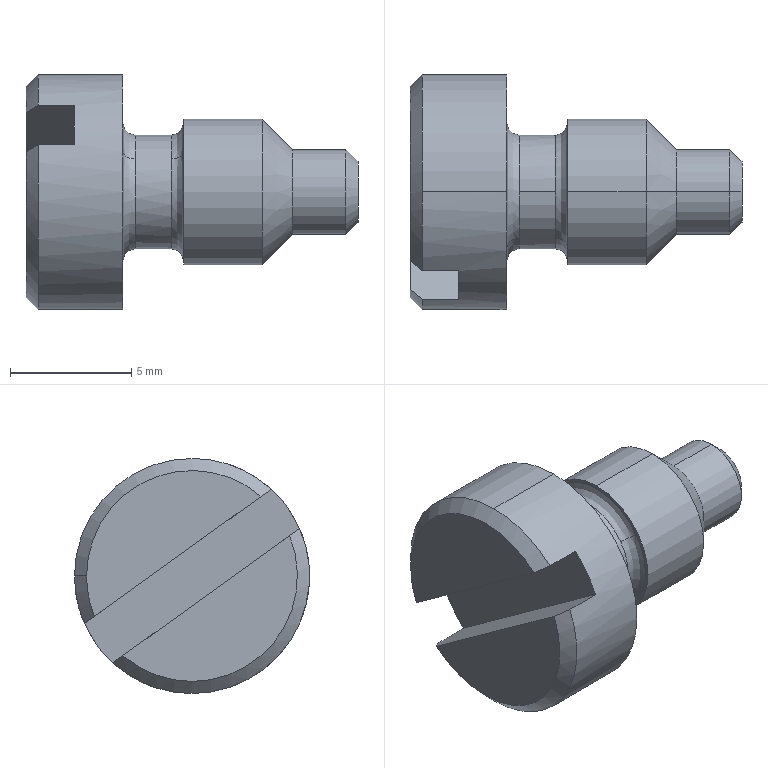Part | SolidWorks | features BaseBody 1 | 1 solid | 27 faces | box 13.7 x 9.7 x 9.7 mm | volume 438.23 mm3 | cylinder 8 | plane 8 | cone 7 | spline 4 | commonest cylinder face diameters 3.5 x2 4.7 x2 6 x2 9.7 x2
STEP:
#1=CARTESIAN_POINT('',(-26.901,-34.08,-0.15));
#2=VERTEX_POINT('',#1);
#3=CARTESIAN_POINT('',(-26.901,-34.08,-9.85));
#4=VERTEX_POINT('',#3);
#5=CARTESIAN_POINT('',(-26.901,-34.08,-5.));
#6=DIRECTION('',(-1.,0.,0.));
#7=DIRECTION('',(0.,0.,1.));
#8=AXIS2_PLACEMENT_3D('',#5,#6,#7);
#9=CIRCLE('',#8,4.85);
#10=EDGE_CURVE('',#2,#4,#9,.T.);
#11=ORIENTED_EDGE('',*,*,#10,.T.);
#12=CARTESIAN_POINT('',(-30.401,-34.08,-9.85));
#13=VERTEX_POINT('',#12);
#14=CARTESIAN_POINT('',(-26.901,-34.08,-9.85));
#15=DIRECTION('',(-1.,0.,0.));
#16=VECTOR('',#15,1000.);
#17=LINE('',#14,#16);
#18=EDGE_CURVE('',#4,#13,#17,.T.);
#19=ORIENTED_EDGE('',*,*,#18,.T.);
#20=CARTESIAN_POINT('',(-30.401,-30.814,-8.586));
#21=VERTEX_POINT('',#20);
#22=CARTESIAN_POINT('',(-30.401,-34.08,-5.));
#23=DIRECTION('',(1.,0.,0.));
#24=DIRECTION('',(0.,0.,1.));
#25=AXIS2_PLACEMENT_3D('',#22,#23,#24);
#26=CIRCLE('',#25,4.85);
#27=EDGE_CURVE('',#13,#21,#26,.T.);
#28=ORIENTED_EDGE('',*,*,#27,.T.);
#29=CARTESIAN_POINT('',(-28.901,-30.814,-8.586));
#30=VERTEX_POINT('',#29);
#31=CARTESIAN_POINT('',(-29.901,-30.814,-8.586));
#32=DIRECTION('',(-1.,0.,0.));
#33=VECTOR('',#32,1000.);
#34=LINE('',#31,#33);
#35=EDGE_CURVE('',#30,#21,#34,.T.);
#36=ORIENTED_EDGE('',*,*,#35,.F.);
#37=CARTESIAN_POINT('',(-28.901,-29.645,-6.963));
#38=VERTEX_POINT('',#37);
#39=CARTESIAN_POINT('',(-28.901,-34.08,-5.));
#40=DIRECTION('',(1.,0.,0.));
#41=DIRECTION('',(0.,0.,1.));
#42=AXIS2_PLACEMENT_3D('',#39,#40,#41);
#43=CIRCLE('',#42,4.85);
#44=EDGE_CURVE('',#30,#38,#43,.T.);
#45=ORIENTED_EDGE('',*,*,#44,.T.);
#46=CARTESIAN_POINT('',(-30.401,-29.645,-6.963));
#47=VERTEX_POINT('',#46);
#48=CARTESIAN_POINT('',(-29.901,-29.645,-6.963));
#49=DIRECTION('',(-1.,0.,0.));
#50=VECTOR('',#49,1000.);
#51=LINE('',#48,#50);
#52=EDGE_CURVE('',#38,#47,#51,.T.);
#53=ORIENTED_EDGE('',*,*,#52,.T.);
#54=CARTESIAN_POINT('',(-30.401,-29.23,-5.));
#55=VERTEX_POINT('',#54);
#56=CARTESIAN_POINT('',(-30.401,-34.08,-5.));
#57=DIRECTION('',(1.,0.,0.));
#58=DIRECTION('',(0.,0.,1.));
#59=AXIS2_PLACEMENT_3D('',#56,#57,#58);
#60=CIRCLE('',#59,4.85);
#61=EDGE_CURVE('',#47,#55,#60,.T.);
#62=ORIENTED_EDGE('',*,*,#61,.T.);
#63=CARTESIAN_POINT('',(-30.401,-34.08,-0.15));
#64=VERTEX_POINT('',#63);
#65=CARTESIAN_POINT('',(-30.401,-34.08,-5.));
#66=DIRECTION('',(1.,0.,0.));
#67=DIRECTION('',(0.,0.,1.));
#68=AXIS2_PLACEMENT_3D('',#65,#66,#67);
#69=CIRCLE('',#68,4.85);
#70=EDGE_CURVE('',#55,#64,#69,.T.);
#71=ORIENTED_EDGE('',*,*,#70,.T.);
#72=CARTESIAN_POINT('',(-26.901,-34.08,-0.15));
#73=DIRECTION('',(-1.,0.,0.));
#74=VECTOR('',#73,1000.);
#75=LINE('',#72,#74);
#76=EDGE_CURVE('',#2,#64,#75,.T.);
#77=ORIENTED_EDGE('',*,*,#76,.F.);
#78=EDGE_LOOP('',(#11,#19,#28,#36,#45,#53,#62,#71,#77));
#79=FACE_OUTER_BOUND('',#78,.T.);
#80=CARTESIAN_POINT('',(-26.901,-34.08,-5.));
#81=DIRECTION('',(-1.,0.,0.));
#82=DIRECTION('',(0.,0.,1.));
#83=AXIS2_PLACEMENT_3D('',#80,#81,#82);
#84=CYLINDRICAL_SURFACE('',#83,4.85);
#85=ADVANCED_FACE('',(#79),#84,.T.);
#86=CARTESIAN_POINT('',(-30.901,-30.061,-6.664));
#87=VERTEX_POINT('',#86);
#88=CARTESIAN_POINT('',(-30.901,-29.73,-5.));
#89=VERTEX_POINT('',#88);
#90=CARTESIAN_POINT('',(-30.901,-34.08,-5.));
#91=DIRECTION('',(1.,0.,0.));
#92=DIRECTION('',(0.,1.,0.));
#93=AXIS2_PLACEMENT_3D('',#90,#91,#92);
#94=CIRCLE('',#93,4.35);
#95=EDGE_CURVE('',#87,#89,#94,.T.);
#96=ORIENTED_EDGE('',*,*,#95,.T.);
#97=CARTESIAN_POINT('',(-30.401,-29.23,-5.));
#98=DIRECTION('',(0.7071,0.7071,0.));
#99=VECTOR('',#98,1000.);
#100=LINE('',#97,#99);
#101=EDGE_CURVE('',#89,#55,#100,.T.);
#102=ORIENTED_EDGE('',*,*,#101,.T.);
#103=ORIENTED_EDGE('',*,*,#61,.F.);
#104=CARTESIAN_POINT('',(-30.401,-29.645,-6.963));
#105=CARTESIAN_POINT('',(-30.568,-29.784,-6.863));
#106=CARTESIAN_POINT('',(-30.735,-29.922,-6.764));
#107=CARTESIAN_POINT('',(-30.901,-30.061,-6.664));
#108=B_SPLINE_CURVE_WITH_KNOTS('',3,(#104,#105,#106,#107),.UNSPECIFIED.,.F.,.F.,(4,4),(0.,0.0007159),.UNSPECIFIED.);
#109=EDGE_CURVE('',#47,#87,#108,.T.);
#110=ORIENTED_EDGE('',*,*,#109,.T.);
#111=EDGE_LOOP('',(#96,#102,#103,#110));
#112=FACE_OUTER_BOUND('',#111,.T.);
#113=CARTESIAN_POINT('',(-30.401,-34.08,-5.));
#114=DIRECTION('',(1.,0.,0.));
#115=DIRECTION('',(0.,1.,0.));
#116=AXIS2_PLACEMENT_3D('',#113,#114,#115);
#117=CONICAL_SURFACE('',#116,4.85,0.7854);
#118=ADVANCED_FACE('',(#112),#117,.T.);
#119=CARTESIAN_POINT('',(-24.901,-32.174,-6.374));
#120=VERTEX_POINT('',#119);
#121=CARTESIAN_POINT('',(-24.901,-34.08,-7.35));
#122=VERTEX_POINT('',#121);
#123=CARTESIAN_POINT('',(-24.901,-34.08,-5.));
#124=DIRECTION('',(-1.,0.,0.));
#125=DIRECTION('',(0.,0.,1.));
#126=AXIS2_PLACEMENT_3D('',#123,#124,#125);
#127=CIRCLE('',#126,2.35);
#128=EDGE_CURVE('',#120,#122,#127,.T.);
#129=ORIENTED_EDGE('',*,*,#128,.T.);
#130=CARTESIAN_POINT('',(-26.401,-34.08,-7.35));
#131=VERTEX_POINT('',#130);
#132=CARTESIAN_POINT('',(-24.901,-34.08,-7.35));
#133=DIRECTION('',(-1.,0.,0.));
#134=VECTOR('',#133,1000.);
#135=LINE('',#132,#134);
#136=EDGE_CURVE('',#122,#131,#135,.T.);
#137=ORIENTED_EDGE('',*,*,#136,.T.);
#138=CARTESIAN_POINT('',(-26.401,-32.174,-6.374));
#139=VERTEX_POINT('',#138);
#140=CARTESIAN_POINT('',(-26.401,-34.08,-5.));
#141=DIRECTION('',(1.,-0.000000001,-0.000000001));
#142=DIRECTION('',(0.,0.8113,-0.5846));
#143=AXIS2_PLACEMENT_3D('',#140,#141,#142);
#144=CIRCLE('',#143,2.35);
#145=EDGE_CURVE('',#131,#139,#144,.T.);
#146=ORIENTED_EDGE('',*,*,#145,.T.);
#147=CARTESIAN_POINT('',(-26.401,-31.73,-5.));
#148=VERTEX_POINT('',#147);
#149=CARTESIAN_POINT('',(-26.401,-34.08,-5.));
#150=DIRECTION('',(1.,0.,0.));
#151=DIRECTION('',(0.,0.,1.));
#152=AXIS2_PLACEMENT_3D('',#149,#150,#151);
#153=CIRCLE('',#152,2.35);
#154=EDGE_CURVE('',#139,#148,#153,.T.);
#155=ORIENTED_EDGE('',*,*,#154,.T.);
#156=CARTESIAN_POINT('',(-26.401,-34.08,-2.65));
#157=VERTEX_POINT('',#156);
#158=CARTESIAN_POINT('',(-26.401,-34.08,-5.));
#159=DIRECTION('',(1.,0.,0.000000001));
#160=DIRECTION('',(0.,-0.8113,0.5846));
#161=AXIS2_PLACEMENT_3D('',#158,#159,#160);
#162=CIRCLE('',#161,2.35);
#163=EDGE_CURVE('',#148,#157,#162,.T.);
#164=ORIENTED_EDGE('',*,*,#163,.T.);
#165=CARTESIAN_POINT('',(-24.901,-34.08,-2.65));
#166=VERTEX_POINT('',#165);
#167=CARTESIAN_POINT('',(-24.901,-34.08,-2.65));
#168=DIRECTION('',(-1.,0.,0.));
#169=VECTOR('',#168,1000.);
#170=LINE('',#167,#169);
#171=EDGE_CURVE('',#166,#157,#170,.T.);
#172=ORIENTED_EDGE('',*,*,#171,.F.);
#173=CARTESIAN_POINT('',(-24.901,-34.08,-5.));
#174=DIRECTION('',(-1.,0.,0.));
#175=DIRECTION('',(0.,0.,1.));
#176=AXIS2_PLACEMENT_3D('',#173,#174,#175);
#177=CIRCLE('',#176,2.35);
#178=EDGE_CURVE('',#166,#120,#177,.T.);
#179=ORIENTED_EDGE('',*,*,#178,.T.);
#180=EDGE_LOOP('',(#129,#137,#146,#155,#164,#172,#179));
#181=FACE_OUTER_BOUND('',#180,.T.);
#182=CARTESIAN_POINT('',(-24.901,-34.08,-5.));
#183=DIRECTION('',(-1.,0.,0.));
#184=DIRECTION('',(0.,0.,1.));
#185=AXIS2_PLACEMENT_3D('',#182,#183,#184);
#186=CYLINDRICAL_SURFACE('',#185,2.35);
#187=ADVANCED_FACE('',(#181),#186,.T.);
#188=CARTESIAN_POINT('',(-21.151,-34.08,-2.));
#189=VERTEX_POINT('',#188);
#190=CARTESIAN_POINT('',(-21.151,-34.08,-8.));
#191=VERTEX_POINT('',#190);
#192=CARTESIAN_POINT('',(-21.151,-34.08,-5.));
#193=DIRECTION('',(-1.,0.,0.));
#194=DIRECTION('',(0.,0.,1.));
#195=AXIS2_PLACEMENT_3D('',#192,#193,#194);
#196=CIRCLE('',#195,3.);
#197=EDGE_CURVE('',#189,#191,#196,.T.);
#198=ORIENTED_EDGE('',*,*,#197,.T.);
#199=CARTESIAN_POINT('',(-24.401,-34.08,-8.));
#200=VERTEX_POINT('',#199);
#201=CARTESIAN_POINT('',(-21.151,-34.08,-8.));
#202=DIRECTION('',(-1.,0.,0.));
#203=VECTOR('',#202,1000.);
#204=LINE('',#201,#203);
#205=EDGE_CURVE('',#191,#200,#204,.T.);
#206=ORIENTED_EDGE('',*,*,#205,.T.);
#207=CARTESIAN_POINT('',(-24.401,-34.08,-2.));
#208=VERTEX_POINT('',#207);
#209=CARTESIAN_POINT('',(-24.401,-34.08,-5.));
#210=DIRECTION('',(1.,0.,0.));
#211=DIRECTION('',(0.,0.,1.));
#212=AXIS2_PLACEMENT_3D('',#209,#210,#211);
#213=CIRCLE('',#212,3.);
#214=EDGE_CURVE('',#200,#208,#213,.T.);
#215=ORIENTED_EDGE('',*,*,#214,.T.);
#216=CARTESIAN_POINT('',(-21.151,-34.08,-2.));
#217=DIRECTION('',(-1.,0.,0.));
#218=VECTOR('',#217,1000.);
#219=LINE('',#216,#218);
#220=EDGE_CURVE('',#189,#208,#219,.T.);
#221=ORIENTED_EDGE('',*,*,#220,.F.);
#222=EDGE_LOOP('',(#198,#206,#215,#221));
#223=FACE_OUTER_BOUND('',#222,.T.);
#224=CARTESIAN_POINT('',(-21.151,-34.08,-5.));
#225=DIRECTION('',(-1.,0.,0.));
#226=DIRECTION('',(0.,0.,1.));
#227=AXIS2_PLACEMENT_3D('',#224,#225,#226);
#228=CYLINDRICAL_SURFACE('',#227,3.);
#229=ADVANCED_FACE('',(#223),#228,.T.);
#230=CARTESIAN_POINT('',(-19.901,-34.08,-3.25));
#231=VERTEX_POINT('',#230);
#232=CARTESIAN_POINT('',(-19.901,-34.08,-6.75));
#233=VERTEX_POINT('',#232);
#234=CARTESIAN_POINT('',(-19.901,-34.08,-5.));
#235=DIRECTION('',(-1.,0.,0.));
#236=DIRECTION('',(0.,0.,1.));
#237=AXIS2_PLACEMENT_3D('',#234,#235,#236);
#238=CIRCLE('',#237,1.75);
#239=EDGE_CURVE('',#231,#233,#238,.T.);
#240=ORIENTED_EDGE('',*,*,#239,.T.);
#241=CARTESIAN_POINT('',(-21.151,-34.08,-8.));
#242=DIRECTION('',(-0.7071,0.,-0.7071));
#243=VECTOR('',#242,1000.);
#244=LINE('',#241,#243);
#245=EDGE_CURVE('',#233,#191,#244,.T.);
#246=ORIENTED_EDGE('',*,*,#245,.T.);
#247=ORIENTED_EDGE('',*,*,#197,.F.);
#248=CARTESIAN_POINT('',(-21.151,-34.08,-2.));
#249=DIRECTION('',(-0.7071,0.,0.7071));
#250=VECTOR('',#249,1000.);
#251=LINE('',#248,#250);
#252=EDGE_CURVE('',#231,#189,#251,.T.);
#253=ORIENTED_EDGE('',*,*,#252,.F.);
#254=EDGE_LOOP('',(#240,#246,#247,#253));
#255=FACE_OUTER_BOUND('',#254,.T.);
#256=CARTESIAN_POINT('',(-21.151,-34.08,-5.));
#257=DIRECTION('',(-1.,0.,0.));
#258=DIRECTION('',(0.,0.,1.));
#259=AXIS2_PLACEMENT_3D('',#256,#257,#258);
#260=CONICAL_SURFACE('',#259,3.,0.7854);
#261=ADVANCED_FACE('',(#255),#260,.T.);
#262=CARTESIAN_POINT('',(-17.701,-34.08,-3.25));
#263=VERTEX_POINT('',#262);
#264=CARTESIAN_POINT('',(-17.701,-34.08,-6.75));
#265=VERTEX_POINT('',#264);
#266=CARTESIAN_POINT('',(-17.701,-34.08,-5.));
#267=DIRECTION('',(-1.,0.,0.));
#268=DIRECTION('',(0.,0.,1.));
#269=AXIS2_PLACEMENT_3D('',#266,#267,#268);
#270=CIRCLE('',#269,1.75);
#271=EDGE_CURVE('',#263,#265,#270,.T.);
#272=ORIENTED_EDGE('',*,*,#271,.T.);
#273=CARTESIAN_POINT('',(-17.701,-34.08,-6.75));
#274=DIRECTION('',(-1.,0.,0.));
#275=VECTOR('',#274,1000.);
#276=LINE('',#273,#275);
#277=EDGE_CURVE('',#265,#233,#276,.T.);
#278=ORIENTED_EDGE('',*,*,#277,.T.);
#279=ORIENTED_EDGE('',*,*,#239,.F.);
#280=CARTESIAN_POINT('',(-17.701,-34.08,-3.25));
#281=DIRECTION('',(-1.,0.,0.));
#282=VECTOR('',#281,1000.);
#283=LINE('',#280,#282);
#284=EDGE_CURVE('',#263,#231,#283,.T.);
#285=ORIENTED_EDGE('',*,*,#284,.F.);
#286=EDGE_LOOP('',(#272,#278,#279,#285));
#287=FACE_OUTER_BOUND('',#286,.T.);
#288=CARTESIAN_POINT('',(-17.701,-34.08,-5.));
#289=DIRECTION('',(-1.,0.,0.));
#290=DIRECTION('',(0.,0.,1.));
#291=AXIS2_PLACEMENT_3D('',#288,#289,#290);
#292=CYLINDRICAL_SURFACE('',#291,1.75);
#293=ADVANCED_FACE('',(#287),#292,.T.);
#294=CARTESIAN_POINT('',(-17.201,-34.08,-3.75));
#295=VERTEX_POINT('',#294);
#296=CARTESIAN_POINT('',(-17.201,-34.08,-6.25));
#297=VERTEX_POINT('',#296);
#298=CARTESIAN_POINT('',(-17.201,-34.08,-5.));
#299=DIRECTION('',(-1.,0.,0.));
#300=DIRECTION('',(0.,0.,1.));
#301=AXIS2_PLACEMENT_3D('',#298,#299,#300);
#302=CIRCLE('',#301,1.25);
#303=EDGE_CURVE('',#295,#297,#302,.T.);
#304=ORIENTED_EDGE('',*,*,#303,.T.);
#305=CARTESIAN_POINT('',(-17.701,-34.08,-6.75));
#306=DIRECTION('',(-0.7071,0.,-0.7071));
#307=VECTOR('',#306,1000.);
#308=LINE('',#305,#307);
#309=EDGE_CURVE('',#297,#265,#308,.T.);
#310=ORIENTED_EDGE('',*,*,#309,.T.);
#311=ORIENTED_EDGE('',*,*,#271,.F.);
#312=CARTESIAN_POINT('',(-17.701,-34.08,-3.25));
#313=DIRECTION('',(-0.7071,0.,0.7071));
#314=VECTOR('',#313,1000.);
#315=LINE('',#312,#314);
#316=EDGE_CURVE('',#295,#263,#315,.T.);
#317=ORIENTED_EDGE('',*,*,#316,.F.);
#318=EDGE_LOOP('',(#304,#310,#311,#317));
#319=FACE_OUTER_BOUND('',#318,.T.);
#320=CARTESIAN_POINT('',(-17.701,-34.08,-5.));
#321=DIRECTION('',(-1.,0.,0.));
#322=DIRECTION('',(0.,0.,1.));
#323=AXIS2_PLACEMENT_3D('',#320,#321,#322);
#324=CONICAL_SURFACE('',#323,1.75,0.7854);
#325=ADVANCED_FACE('',(#319),#324,.T.);
#326=ORIENTED_EDGE('',*,*,#18,.F.);
#327=CARTESIAN_POINT('',(-26.901,-34.08,-5.));
#328=DIRECTION('',(-1.,0.,0.));
#329=DIRECTION('',(0.,0.,1.));
#330=AXIS2_PLACEMENT_3D('',#327,#328,#329);
#331=CIRCLE('',#330,4.85);
#332=EDGE_CURVE('',#4,#2,#331,.T.);
#333=ORIENTED_EDGE('',*,*,#332,.T.);
#334=ORIENTED_EDGE('',*,*,#76,.T.);
#335=CARTESIAN_POINT('',(-30.401,-37.346,-1.414));
#336=VERTEX_POINT('',#335);
#337=CARTESIAN_POINT('',(-30.401,-34.08,-5.));
#338=DIRECTION('',(1.,0.,0.));
#339=DIRECTION('',(0.,0.,1.));
#340=AXIS2_PLACEMENT_3D('',#337,#338,#339);
#341=CIRCLE('',#340,4.85);
#342=EDGE_CURVE('',#64,#336,#341,.T.);
#343=ORIENTED_EDGE('',*,*,#342,.T.);
#344=CARTESIAN_POINT('',(-28.901,-37.346,-1.414));
#345=VERTEX_POINT('',#344);
#346=CARTESIAN_POINT('',(-29.901,-37.346,-1.414));
#347=DIRECTION('',(1.,0.,0.));
#348=VECTOR('',#347,1000.);
#349=LINE('',#346,#348);
#350=EDGE_CURVE('',#336,#345,#349,.T.);
#351=ORIENTED_EDGE('',*,*,#350,.T.);
#352=CARTESIAN_POINT('',(-28.901,-38.515,-3.037));
#353=VERTEX_POINT('',#352);
#354=CARTESIAN_POINT('',(-28.901,-34.08,-5.));
#355=DIRECTION('',(1.,0.,0.));
#356=DIRECTION('',(0.,0.,1.));
#357=AXIS2_PLACEMENT_3D('',#354,#355,#356);
#358=CIRCLE('',#357,4.85);
#359=EDGE_CURVE('',#345,#353,#358,.T.);
#360=ORIENTED_EDGE('',*,*,#359,.T.);
#361=CARTESIAN_POINT('',(-30.401,-38.515,-3.037));
#362=VERTEX_POINT('',#361);
#363=CARTESIAN_POINT('',(-29.901,-38.515,-3.037));
#364=DIRECTION('',(1.,0.,0.));
#365=VECTOR('',#364,1000.);
#366=LINE('',#363,#365);
#367=EDGE_CURVE('',#362,#353,#366,.T.);
#368=ORIENTED_EDGE('',*,*,#367,.F.);
#369=CARTESIAN_POINT('',(-30.401,-34.08,-5.));
#370=DIRECTION('',(1.,0.,0.));
#371=DIRECTION('',(0.,0.,1.));
#372=AXIS2_PLACEMENT_3D('',#369,#370,#371);
#373=CIRCLE('',#372,4.85);
#374=EDGE_CURVE('',#362,#13,#373,.T.);
#375=ORIENTED_EDGE('',*,*,#374,.T.);
#376=EDGE_LOOP('',(#326,#333,#334,#343,#351,#360,#368,#375));
#377=FACE_OUTER_BOUND('',#376,.T.);
#378=CARTESIAN_POINT('',(-26.901,-34.08,-5.));
#379=DIRECTION('',(-1.,0.,0.));
#380=DIRECTION('',(0.,0.,1.));
#381=AXIS2_PLACEMENT_3D('',#378,#379,#380);
#382=CYLINDRICAL_SURFACE('',#381,4.85);
#383=ADVANCED_FACE('',(#377),#382,.T.);
#384=CARTESIAN_POINT('',(-26.901,-31.768,-6.666));
#385=VERTEX_POINT('',#384);
#386=CARTESIAN_POINT('',(-26.901,-36.392,-3.334));
#387=VERTEX_POINT('',#386);
#388=CARTESIAN_POINT('',(-26.901,-31.768,-6.666));
#389=CARTESIAN_POINT('',(-26.901,-31.878,-6.818));
#390=CARTESIAN_POINT('',(-26.901,-32.061,-7.026));
#391=CARTESIAN_POINT('',(-26.901,-32.307,-7.235));
#392=CARTESIAN_POINT('',(-26.901,-32.419,-7.317));
#393=CARTESIAN_POINT('',(-26.901,-32.496,-7.369));
#394=CARTESIAN_POINT('',(-26.901,-32.534,-7.394));
#395=CARTESIAN_POINT('',(-26.901,-32.738,-7.522));
#396=CARTESIAN_POINT('',(-26.901,-32.993,-7.647));
#397=CARTESIAN_POINT('',(-26.901,-33.309,-7.747));
#398=CARTESIAN_POINT('',(-26.901,-33.448,-7.78));
#399=CARTESIAN_POINT('',(-26.901,-33.541,-7.799));
#400=CARTESIAN_POINT('',(-26.901,-33.591,-7.808));
#401=CARTESIAN_POINT('',(-26.901,-33.819,-7.844));
#402=CARTESIAN_POINT('',(-26.901,-34.091,-7.861));
#403=CARTESIAN_POINT('',(-26.901,-34.408,-7.834));
#404=CARTESIAN_POINT('',(-26.901,-34.543,-7.813));
#405=CARTESIAN_POINT('',(-26.901,-34.634,-7.796));
#406=CARTESIAN_POINT('',(-26.901,-34.677,-7.787));
#407=CARTESIAN_POINT('',(-26.901,-35.095,-7.69));
#408=CARTESIAN_POINT('',(-26.901,-35.437,-7.535));
#409=CARTESIAN_POINT('',(-26.901,-35.901,-7.201));
#410=CARTESIAN_POINT('',(-26.901,-36.113,-7.014));
#411=CARTESIAN_POINT('',(-26.901,-36.323,-6.763));
#412=CARTESIAN_POINT('',(-26.901,-36.406,-6.648));
#413=CARTESIAN_POINT('',(-26.901,-36.459,-6.57));
#414=CARTESIAN_POINT('',(-26.901,-36.486,-6.528));
#415=CARTESIAN_POINT('',(-26.901,-36.607,-6.332));
#416=CARTESIAN_POINT('',(-26.901,-36.727,-6.086));
#417=CARTESIAN_POINT('',(-26.901,-36.823,-5.783));
#418=CARTESIAN_POINT('',(-26.901,-36.856,-5.65));
#419=CARTESIAN_POINT('',(-26.901,-36.875,-5.56));
#420=CARTESIAN_POINT('',(-26.901,-36.883,-5.517));
#421=CARTESIAN_POINT('',(-26.901,-36.923,-5.28));
#422=CARTESIAN_POINT('',(-26.901,-36.942,-4.996));
#423=CARTESIAN_POINT('',(-26.901,-36.914,-4.666));
#424=CARTESIAN_POINT('',(-26.901,-36.891,-4.525));
#425=CARTESIAN_POINT('',(-26.901,-36.873,-4.431));
#426=CARTESIAN_POINT('',(-26.901,-36.863,-4.383));
#427=CARTESIAN_POINT('',(-26.901,-36.765,-3.973));
#428=CARTESIAN_POINT('',(-26.901,-36.612,-3.638));
#429=CARTESIAN_POINT('',(-26.901,-36.392,-3.334));
#430=B_SPLINE_CURVE_WITH_KNOTS('',3,(#388,#389,#390,#391,#392,#393,#394,#395,#396,#397,#398,#399,#400,#401,#402,#403,#404,#405,#406,#407,#408,#409,#410,#411,#412,#413,#414,#415,#416,#417,#418,#419,#420,#421,#422,#423,#424,#425,#426,#427,#428,#429),.UNSPECIFIED.,.F.,.F.,(4,1,1,2,2,1,1,2,2,1,1,2,2,2,1,1,2,2,1,1,2,2,1,1,2,2,4),(0.,0.0625,0.09375,0.1094,0.125,0.1875,0.2187,0.2344,0.25,0.3125,0.3438,0.3594,0.375,0.5,0.5625,0.5937,0.6094,0.625,0.6875,0.7187,0.7344,0.75,0.8125,0.8437,0.8594,0.875,1.),.UNSPECIFIED.);
#431=EDGE_CURVE('',#385,#387,#430,.T.);
#432=ORIENTED_EDGE('',*,*,#431,.T.);
#433=CARTESIAN_POINT('',(-26.901,-36.392,-3.334));
#434=CARTESIAN_POINT('',(-26.901,-36.287,-3.187));
#435=CARTESIAN_POINT('',(-26.901,-36.11,-2.985));
#436=CARTESIAN_POINT('',(-26.901,-35.874,-2.782));
#437=CARTESIAN_POINT('',(-26.901,-35.748,-2.688));
#438=CARTESIAN_POINT('',(-26.901,-35.692,-2.65));
#439=CARTESIAN_POINT('',(-26.901,-35.655,-2.624));
#440=CARTESIAN_POINT('',(-26.901,-35.637,-2.613));
#441=CARTESIAN_POINT('',(-26.901,-35.286,-2.388));
#442=CARTESIAN_POINT('',(-26.901,-34.925,-2.25));
#443=CARTESIAN_POINT('',(-26.901,-34.343,-2.155));
#444=CARTESIAN_POINT('',(-26.901,-34.053,-2.138));
#445=CARTESIAN_POINT('',(-26.901,-33.717,-2.17));
#446=CARTESIAN_POINT('',(-26.901,-33.549,-2.199));
#447=CARTESIAN_POINT('',(-26.901,-33.478,-2.214));
#448=CARTESIAN_POINT('',(-26.901,-33.43,-2.225));
#449=CARTESIAN_POINT('',(-26.901,-33.404,-2.231));
#450=CARTESIAN_POINT('',(-26.901,-33.031,-2.325));
#451=CARTESIAN_POINT('',(-26.901,-32.708,-2.476));
#452=CARTESIAN_POINT('',(-26.901,-32.267,-2.794));
#453=CARTESIAN_POINT('',(-26.901,-32.065,-2.97));
#454=CARTESIAN_POINT('',(-26.901,-31.862,-3.206));
#455=CARTESIAN_POINT('',(-26.901,-31.768,-3.332));
#456=CARTESIAN_POINT('',(-26.901,-31.73,-3.388));
#457=CARTESIAN_POINT('',(-26.901,-31.705,-3.425));
#458=CARTESIAN_POINT('',(-26.901,-31.693,-3.443));
#459=CARTESIAN_POINT('',(-26.901,-31.468,-3.794));
#460=CARTESIAN_POINT('',(-26.901,-31.33,-4.155));
#461=CARTESIAN_POINT('',(-26.901,-31.235,-4.737));
#462=CARTESIAN_POINT('',(-26.901,-31.218,-5.027));
#463=CARTESIAN_POINT('',(-26.901,-31.25,-5.363));
#464=CARTESIAN_POINT('',(-26.901,-31.279,-5.531));
#465=CARTESIAN_POINT('',(-26.901,-31.294,-5.602));
#466=CARTESIAN_POINT('',(-26.901,-31.305,-5.65));
#467=CARTESIAN_POINT('',(-26.901,-31.311,-5.676));
#468=CARTESIAN_POINT('',(-26.901,-31.406,-6.049));
#469=CARTESIAN_POINT('',(-26.901,-31.556,-6.372));
#470=CARTESIAN_POINT('',(-26.901,-31.768,-6.666));
#471=B_SPLINE_CURVE_WITH_KNOTS('',3,(#433,#434,#435,#436,#437,#438,#439,#440,#441,#442,#443,#444,#445,#446,#447,#448,#449,#450,#451,#452,#453,#454,#455,#456,#457,#458,#459,#460,#461,#462,#463,#464,#465,#466,#467,#468,#469,#470),.UNSPECIFIED.,.F.,.F.,(4,1,1,1,2,2,2,1,1,1,2,2,2,1,1,1,2,2,2,1,1,1,2,2,4),(0.,0.0625,0.09375,0.1094,0.1172,0.125,0.25,0.3125,0.3438,0.3594,0.3672,0.375,0.5,0.5625,0.5937,0.6094,0.6172,0.625,0.75,0.8125,0.8437,0.8594,0.8672,0.875,1.),.UNSPECIFIED.);
#472=EDGE_CURVE('',#387,#385,#471,.T.);
#473=ORIENTED_EDGE('',*,*,#472,.T.);
#474=EDGE_LOOP('',(#432,#473));
#475=FACE_BOUND('',#474,.T.);
#476=ORIENTED_EDGE('',*,*,#10,.F.);
#477=ORIENTED_EDGE('',*,*,#332,.F.);
#478=EDGE_LOOP('',(#476,#477));
#479=FACE_OUTER_BOUND('',#478,.T.);
#480=CARTESIAN_POINT('',(-26.901,-34.08,-5.));
#481=DIRECTION('',(1.,0.,0.));
#482=DIRECTION('',(0.,0.,-1.));
#483=AXIS2_PLACEMENT_3D('',#480,#481,#482);
#484=PLANE('',#483);
#485=ADVANCED_FACE('',(#475,#479),#484,.T.);
#486=ORIENTED_EDGE('',*,*,#101,.F.);
#487=CARTESIAN_POINT('',(-30.901,-36.93,-1.714));
#488=VERTEX_POINT('',#487);
#489=CARTESIAN_POINT('',(-30.901,-34.08,-5.));
#490=DIRECTION('',(1.,0.,0.));
#491=DIRECTION('',(0.,1.,0.));
#492=AXIS2_PLACEMENT_3D('',#489,#490,#491);
#493=CIRCLE('',#492,4.35);
#494=EDGE_CURVE('',#89,#488,#493,.T.);
#495=ORIENTED_EDGE('',*,*,#494,.T.);
#496=CARTESIAN_POINT('',(-30.901,-36.93,-1.714));
#497=CARTESIAN_POINT('',(-30.735,-37.069,-1.614));
#498=CARTESIAN_POINT('',(-30.568,-37.208,-1.514));
#499=CARTESIAN_POINT('',(-30.401,-37.346,-1.414));
#500=B_SPLINE_CURVE_WITH_KNOTS('',3,(#496,#497,#498,#499),.UNSPECIFIED.,.F.,.F.,(4,4),(0.,0.0007159),.UNSPECIFIED.);
#501=EDGE_CURVE('',#488,#336,#500,.T.);
#502=ORIENTED_EDGE('',*,*,#501,.T.);
#503=ORIENTED_EDGE('',*,*,#342,.F.);
#504=ORIENTED_EDGE('',*,*,#70,.F.);
#505=EDGE_LOOP('',(#486,#495,#502,#503,#504));
#506=FACE_OUTER_BOUND('',#505,.T.);
#507=CARTESIAN_POINT('',(-30.401,-34.08,-5.));
#508=DIRECTION('',(1.,0.,0.));
#509=DIRECTION('',(0.,1.,0.));
#510=AXIS2_PLACEMENT_3D('',#507,#508,#509);
#511=CONICAL_SURFACE('',#510,4.85,0.7854);
#512=ADVANCED_FACE('',(#506),#511,.T.);
#513=ORIENTED_EDGE('',*,*,#359,.F.);
#514=CARTESIAN_POINT('',(-28.901,-29.645,-6.963));
#515=DIRECTION('',(0.,-0.8113,0.5846));
#516=VECTOR('',#515,1000.);
#517=LINE('',#514,#516);
#518=EDGE_CURVE('',#38,#345,#517,.T.);
#519=ORIENTED_EDGE('',*,*,#518,.F.);
#520=ORIENTED_EDGE('',*,*,#44,.F.);
#521=CARTESIAN_POINT('',(-28.901,-38.515,-3.037));
#522=DIRECTION('',(0.,0.8113,-0.5846));
#523=VECTOR('',#522,1000.);
#524=LINE('',#521,#523);
#525=EDGE_CURVE('',#353,#30,#524,.T.);
#526=ORIENTED_EDGE('',*,*,#525,.F.);
#527=EDGE_LOOP('',(#513,#519,#520,#526));
#528=FACE_OUTER_BOUND('',#527,.T.);
#529=CARTESIAN_POINT('',(-28.901,-34.08,-5.));
#530=DIRECTION('',(1.,0.,0.));
#531=DIRECTION('',(0.,0.,-1.));
#532=AXIS2_PLACEMENT_3D('',#529,#530,#531);
#533=PLANE('',#532);
#534=ADVANCED_FACE('',(#528),#533,.F.);
#535=ORIENTED_EDGE('',*,*,#374,.F.);
#536=CARTESIAN_POINT('',(-30.901,-38.099,-3.336));
#537=VERTEX_POINT('',#536);
#538=CARTESIAN_POINT('',(-30.401,-38.515,-3.037));
#539=CARTESIAN_POINT('',(-30.568,-38.377,-3.137));
#540=CARTESIAN_POINT('',(-30.735,-38.238,-3.236));
#541=CARTESIAN_POINT('',(-30.901,-38.099,-3.336));
#542=B_SPLINE_CURVE_WITH_KNOTS('',3,(#538,#539,#540,#541),.UNSPECIFIED.,.F.,.F.,(4,4),(0.,0.0007159),.UNSPECIFIED.);
#543=EDGE_CURVE('',#362,#537,#542,.T.);
#544=ORIENTED_EDGE('',*,*,#543,.T.);
#545=CARTESIAN_POINT('',(-30.901,-31.23,-8.286));
#546=VERTEX_POINT('',#545);
#547=CARTESIAN_POINT('',(-30.901,-34.08,-5.));
#548=DIRECTION('',(1.,0.,0.));
#549=DIRECTION('',(0.,1.,0.));
#550=AXIS2_PLACEMENT_3D('',#547,#548,#549);
#551=CIRCLE('',#550,4.35);
#552=EDGE_CURVE('',#537,#546,#551,.T.);
#553=ORIENTED_EDGE('',*,*,#552,.T.);
#554=CARTESIAN_POINT('',(-30.901,-31.23,-8.286));
#555=CARTESIAN_POINT('',(-30.735,-31.091,-8.386));
#556=CARTESIAN_POINT('',(-30.568,-30.953,-8.486));
#557=CARTESIAN_POINT('',(-30.401,-30.814,-8.586));
#558=B_SPLINE_CURVE_WITH_KNOTS('',3,(#554,#555,#556,#557),.UNSPECIFIED.,.F.,.F.,(4,4),(0.,0.0007159),.UNSPECIFIED.);
#559=EDGE_CURVE('',#546,#21,#558,.T.);
#560=ORIENTED_EDGE('',*,*,#559,.T.);
#561=ORIENTED_EDGE('',*,*,#27,.F.);
#562=EDGE_LOOP('',(#535,#544,#553,#560,#561));
#563=FACE_OUTER_BOUND('',#562,.T.);
#564=CARTESIAN_POINT('',(-30.401,-34.08,-5.));
#565=DIRECTION('',(1.,0.,0.));
#566=DIRECTION('',(0.,1.,0.));
#567=AXIS2_PLACEMENT_3D('',#564,#565,#566);
#568=CONICAL_SURFACE('',#567,4.85,0.7854);
#569=ADVANCED_FACE('',(#563),#568,.T.);
#570=ORIENTED_EDGE('',*,*,#154,.F.);
#571=CARTESIAN_POINT('',(-26.401,-31.768,-6.666));
#572=DIRECTION('',(-0.000000001,0.5846,0.8113));
#573=DIRECTION('',(0.,0.8113,-0.5846));
#574=AXIS2_PLACEMENT_3D('',#571,#572,#573);
#575=CIRCLE('',#574,0.5);
#576=EDGE_CURVE('',#385,#139,#575,.T.);
#577=ORIENTED_EDGE('',*,*,#576,.F.);
#578=ORIENTED_EDGE('',*,*,#472,.F.);
#579=CARTESIAN_POINT('',(-26.401,-35.987,-3.626));
#580=VERTEX_POINT('',#579);
#581=CARTESIAN_POINT('',(-26.401,-36.392,-3.334));
#582=DIRECTION('',(0.000000001,0.5846,0.8113));
#583=DIRECTION('',(0.,-0.8113,0.5846));
#584=AXIS2_PLACEMENT_3D('',#581,#582,#583);
#585=CIRCLE('',#584,0.5);
#586=EDGE_CURVE('',#580,#387,#585,.T.);
#587=ORIENTED_EDGE('',*,*,#586,.F.);
#588=CARTESIAN_POINT('',(-26.401,-34.08,-5.));
#589=DIRECTION('',(1.,0.,0.000000001));
#590=DIRECTION('',(0.,-0.8113,0.5846));
#591=AXIS2_PLACEMENT_3D('',#588,#589,#590);
#592=CIRCLE('',#591,2.35);
#593=EDGE_CURVE('',#157,#580,#592,.T.);
#594=ORIENTED_EDGE('',*,*,#593,.F.);
#595=ORIENTED_EDGE('',*,*,#163,.F.);
#596=EDGE_LOOP('',(#570,#577,#578,#587,#594,#595));
#597=FACE_OUTER_BOUND('',#596,.T.);
#598=CARTESIAN_POINT('',(-26.401,-35.987,-3.626));
#599=CARTESIAN_POINT('',(-26.401,-35.182,-2.509));
#600=CARTESIAN_POINT('',(-26.401,-33.823,-2.289));
#601=CARTESIAN_POINT('',(-26.401,-32.706,-3.093));
#602=CARTESIAN_POINT('',(-26.401,-31.59,-3.898));
#603=CARTESIAN_POINT('',(-26.401,-31.369,-5.257));
#604=CARTESIAN_POINT('',(-26.401,-32.174,-6.374));
#605=CARTESIAN_POINT('',(-26.694,-35.987,-3.626));
#606=CARTESIAN_POINT('',(-26.694,-35.182,-2.509));
#607=CARTESIAN_POINT('',(-26.694,-33.823,-2.289));
#608=CARTESIAN_POINT('',(-26.694,-32.706,-3.093));
#609=CARTESIAN_POINT('',(-26.694,-31.59,-3.898));
#610=CARTESIAN_POINT('',(-26.694,-31.369,-5.257));
#611=CARTESIAN_POINT('',(-26.694,-32.174,-6.374));
#612=CARTESIAN_POINT('',(-26.901,-36.155,-3.505));
#613=CARTESIAN_POINT('',(-26.901,-35.279,-2.29));
#614=CARTESIAN_POINT('',(-26.901,-33.801,-2.05));
#615=CARTESIAN_POINT('',(-26.901,-32.585,-2.925));
#616=CARTESIAN_POINT('',(-26.901,-31.37,-3.801));
#617=CARTESIAN_POINT('',(-26.901,-31.13,-5.28));
#618=CARTESIAN_POINT('',(-26.901,-32.006,-6.495));
#619=CARTESIAN_POINT('',(-26.901,-36.392,-3.334));
#620=CARTESIAN_POINT('',(-26.901,-35.416,-1.979));
#621=CARTESIAN_POINT('',(-26.901,-33.769,-1.712));
#622=CARTESIAN_POINT('',(-26.901,-32.414,-2.688));
#623=CARTESIAN_POINT('',(-26.901,-31.06,-3.664));
#624=CARTESIAN_POINT('',(-26.901,-30.792,-5.312));
#625=CARTESIAN_POINT('',(-26.901,-31.768,-6.666));
#626=(BOUNDED_SURFACE()B_SPLINE_SURFACE(3,3,((#598,#599,#600,#601,#602,#603,#604),(#605,#606,#607,#608,#609,#610,#611),(#612,#613,#614,#615,#616,#617,#618),(#619,#620,#621,#622,#623,#624,#625)),.UNSPECIFIED.,.F.,.F.,.T.)B_SPLINE_SURFACE_WITH_KNOTS((4,4),(4,3,4),(0.,1.),(0.,0.5,1.),.UNSPECIFIED.)GEOMETRIC_REPRESENTATION_ITEM()RATIONAL_B_SPLINE_SURFACE(((1.,0.8047,0.8047,1.,0.8047,0.8047,1.),(0.8047,0.6476,0.6476,0.8047,0.6476,0.6476,0.8047),(0.8047,0.6476,0.6476,0.8047,0.6476,0.6476,0.8047),(1.,0.8047,0.8047,1.,0.8047,0.8047,1.)))REPRESENTATION_ITEM('')SURFACE());
#627=ADVANCED_FACE('',(#597),#626,.F.);
#628=ORIENTED_EDGE('',*,*,#431,.F.);
#629=ORIENTED_EDGE('',*,*,#576,.T.);
#630=ORIENTED_EDGE('',*,*,#145,.F.);
#631=CARTESIAN_POINT('',(-26.401,-34.08,-5.));
#632=DIRECTION('',(1.,-0.000000001,-0.000000001));
#633=DIRECTION('',(0.,0.8113,-0.5846));
#634=AXIS2_PLACEMENT_3D('',#631,#632,#633);
#635=CIRCLE('',#634,2.35);
#636=EDGE_CURVE('',#580,#131,#635,.T.);
#637=ORIENTED_EDGE('',*,*,#636,.F.);
#638=ORIENTED_EDGE('',*,*,#586,.T.);
#639=EDGE_LOOP('',(#628,#629,#630,#637,#638));
#640=FACE_OUTER_BOUND('',#639,.T.);
#641=CARTESIAN_POINT('',(-26.401,-32.174,-6.374));
#642=CARTESIAN_POINT('',(-26.401,-32.978,-7.491));
#643=CARTESIAN_POINT('',(-26.401,-34.337,-7.711));
#644=CARTESIAN_POINT('',(-26.401,-35.454,-6.907));
#645=CARTESIAN_POINT('',(-26.401,-36.571,-6.102));
#646=CARTESIAN_POINT('',(-26.401,-36.792,-4.743));
#647=CARTESIAN_POINT('',(-26.401,-35.987,-3.626));
#648=CARTESIAN_POINT('',(-26.694,-32.174,-6.374));
#649=CARTESIAN_POINT('',(-26.694,-32.978,-7.491));
#650=CARTESIAN_POINT('',(-26.694,-34.337,-7.711));
#651=CARTESIAN_POINT('',(-26.694,-35.454,-6.907));
#652=CARTESIAN_POINT('',(-26.694,-36.571,-6.102));
#653=CARTESIAN_POINT('',(-26.694,-36.792,-4.743));
#654=CARTESIAN_POINT('',(-26.694,-35.987,-3.626));
#655=CARTESIAN_POINT('',(-26.901,-32.006,-6.495));
#656=CARTESIAN_POINT('',(-26.901,-32.881,-7.71));
#657=CARTESIAN_POINT('',(-26.901,-34.36,-7.95));
#658=CARTESIAN_POINT('',(-26.901,-35.575,-7.075));
#659=CARTESIAN_POINT('',(-26.901,-36.79,-6.199));
#660=CARTESIAN_POINT('',(-26.901,-37.031,-4.72));
#661=CARTESIAN_POINT('',(-26.901,-36.155,-3.505));
#662=CARTESIAN_POINT('',(-26.901,-31.768,-6.666));
#663=CARTESIAN_POINT('',(-26.901,-32.744,-8.021));
#664=CARTESIAN_POINT('',(-26.901,-34.392,-8.288));
#665=CARTESIAN_POINT('',(-26.901,-35.746,-7.312));
#666=CARTESIAN_POINT('',(-26.901,-37.101,-6.336));
#667=CARTESIAN_POINT('',(-26.901,-37.368,-4.688));
#668=CARTESIAN_POINT('',(-26.901,-36.392,-3.334));
#669=(BOUNDED_SURFACE()B_SPLINE_SURFACE(3,3,((#641,#642,#643,#644,#645,#646,#647),(#648,#649,#650,#651,#652,#653,#654),(#655,#656,#657,#658,#659,#660,#661),(#662,#663,#664,#665,#666,#667,#668)),.UNSPECIFIED.,.F.,.F.,.F.)B_SPLINE_SURFACE_WITH_KNOTS((4,4),(4,3,4),(0.,1.),(0.,0.5,1.),.UNSPECIFIED.)GEOMETRIC_REPRESENTATION_ITEM()RATIONAL_B_SPLINE_SURFACE(((1.,0.8047,0.8047,1.,0.8047,0.8047,1.),(0.8047,0.6476,0.6476,0.8047,0.6476,0.6476,0.8047),(0.8047,0.6476,0.6476,0.8047,0.6476,0.6476,0.8047),(1.,0.8047,0.8047,1.,0.8047,0.8047,1.)))REPRESENTATION_ITEM('')SURFACE());
#670=ADVANCED_FACE('',(#640),#669,.F.);
#671=CARTESIAN_POINT('',(-30.901,-36.93,-1.714));
#672=DIRECTION('',(0.,0.8113,-0.5846));
#673=VECTOR('',#672,1000.);
#674=LINE('',#671,#673);
#675=EDGE_CURVE('',#488,#87,#674,.T.);
#676=ORIENTED_EDGE('',*,*,#675,.F.);
#677=ORIENTED_EDGE('',*,*,#494,.F.);
#678=ORIENTED_EDGE('',*,*,#95,.F.);
#679=EDGE_LOOP('',(#676,#677,#678));
#680=FACE_OUTER_BOUND('',#679,.T.);
#681=CARTESIAN_POINT('',(-30.901,-33.328,-3.655));
#682=DIRECTION('',(1.,0.,0.));
#683=DIRECTION('',(0.,0.,-1.));
#684=AXIS2_PLACEMENT_3D('',#681,#682,#683);
#685=PLANE('',#684);
#686=ADVANCED_FACE('',(#680),#685,.F.);
#687=ORIENTED_EDGE('',*,*,#367,.T.);
#688=ORIENTED_EDGE('',*,*,#525,.T.);
#689=ORIENTED_EDGE('',*,*,#35,.T.);
#690=ORIENTED_EDGE('',*,*,#559,.F.);
#691=CARTESIAN_POINT('',(-30.901,-34.665,-5.811));
#692=DIRECTION('',(0.,-0.8113,0.5846));
#693=VECTOR('',#692,1000.);
#694=LINE('',#691,#693);
#695=EDGE_CURVE('',#546,#537,#694,.T.);
#696=ORIENTED_EDGE('',*,*,#695,.T.);
#697=ORIENTED_EDGE('',*,*,#543,.F.);
#698=EDGE_LOOP('',(#687,#688,#689,#690,#696,#697));
#699=FACE_OUTER_BOUND('',#698,.T.);
#700=CARTESIAN_POINT('',(-29.901,-34.665,-5.811));
#701=DIRECTION('',(0.,0.5846,0.8113));
#702=DIRECTION('',(0.,-0.8113,0.5846));
#703=AXIS2_PLACEMENT_3D('',#700,#701,#702);
#704=PLANE('',#703);
#705=ADVANCED_FACE('',(#699),#704,.T.);
#706=ORIENTED_EDGE('',*,*,#350,.F.);
#707=ORIENTED_EDGE('',*,*,#501,.F.);
#708=ORIENTED_EDGE('',*,*,#675,.T.);
#709=ORIENTED_EDGE('',*,*,#109,.F.);
#710=ORIENTED_EDGE('',*,*,#52,.F.);
#711=ORIENTED_EDGE('',*,*,#518,.T.);
#712=EDGE_LOOP('',(#706,#707,#708,#709,#710,#711));
#713=FACE_OUTER_BOUND('',#712,.T.);
#714=CARTESIAN_POINT('',(-29.901,-33.496,-4.189));
#715=DIRECTION('',(0.,0.5846,0.8113));
#716=DIRECTION('',(0.,-0.8113,0.5846));
#717=AXIS2_PLACEMENT_3D('',#714,#715,#716);
#718=PLANE('',#717);
#719=ADVANCED_FACE('',(#713),#718,.F.);
#720=ORIENTED_EDGE('',*,*,#552,.F.);
#721=ORIENTED_EDGE('',*,*,#695,.F.);
#722=EDGE_LOOP('',(#720,#721));
#723=FACE_OUTER_BOUND('',#722,.T.);
#724=CARTESIAN_POINT('',(-30.901,-34.831,-6.343));
#725=DIRECTION('',(1.,0.,0.));
#726=DIRECTION('',(0.,0.,-1.));
#727=AXIS2_PLACEMENT_3D('',#724,#725,#726);
#728=PLANE('',#727);
#729=ADVANCED_FACE('',(#723),#728,.F.);
#730=ORIENTED_EDGE('',*,*,#136,.F.);
#731=CARTESIAN_POINT('',(-24.901,-36.43,-5.));
#732=VERTEX_POINT('',#731);
#733=CARTESIAN_POINT('',(-24.901,-34.08,-5.));
#734=DIRECTION('',(-1.,0.,0.));
#735=DIRECTION('',(0.,0.,1.));
#736=AXIS2_PLACEMENT_3D('',#733,#734,#735);
#737=CIRCLE('',#736,2.35);
#738=EDGE_CURVE('',#122,#732,#737,.T.);
#739=ORIENTED_EDGE('',*,*,#738,.T.);
#740=CARTESIAN_POINT('',(-24.901,-35.987,-3.626));
#741=VERTEX_POINT('',#740);
#742=CARTESIAN_POINT('',(-24.901,-34.08,-5.));
#743=DIRECTION('',(-1.,0.,-0.000000001));
#744=DIRECTION('',(0.,-0.8113,0.5846));
#745=AXIS2_PLACEMENT_3D('',#742,#743,#744);
#746=CIRCLE('',#745,2.35);
#747=EDGE_CURVE('',#732,#741,#746,.T.);
#748=ORIENTED_EDGE('',*,*,#747,.T.);
#749=CARTESIAN_POINT('',(-24.901,-34.08,-5.));
#750=DIRECTION('',(-1.,0.,0.));
#751=DIRECTION('',(0.,0.,1.));
#752=AXIS2_PLACEMENT_3D('',#749,#750,#751);
#753=CIRCLE('',#752,2.35);
#754=EDGE_CURVE('',#741,#166,#753,.T.);
#755=ORIENTED_EDGE('',*,*,#754,.T.);
#756=ORIENTED_EDGE('',*,*,#171,.T.);
#757=ORIENTED_EDGE('',*,*,#593,.T.);
#758=ORIENTED_EDGE('',*,*,#636,.T.);
#759=EDGE_LOOP('',(#730,#739,#748,#755,#756,#757,#758));
#760=FACE_OUTER_BOUND('',#759,.T.);
#761=CARTESIAN_POINT('',(-24.901,-34.08,-5.));
#762=DIRECTION('',(-1.,0.,0.));
#763=DIRECTION('',(0.,0.,1.));
#764=AXIS2_PLACEMENT_3D('',#761,#762,#763);
#765=CYLINDRICAL_SURFACE('',#764,2.35);
#766=ADVANCED_FACE('',(#760),#765,.T.);
#767=CARTESIAN_POINT('',(-24.401,-31.768,-6.666));
#768=VERTEX_POINT('',#767);
#769=CARTESIAN_POINT('',(-24.901,-31.768,-6.666));
#770=DIRECTION('',(0.000000001,0.5846,0.8113));
#771=DIRECTION('',(0.,0.8113,-0.5846));
#772=AXIS2_PLACEMENT_3D('',#769,#770,#771);
#773=CIRCLE('',#772,0.5);
#774=EDGE_CURVE('',#120,#768,#773,.T.);
#775=ORIENTED_EDGE('',*,*,#774,.F.);
#776=ORIENTED_EDGE('',*,*,#178,.F.);
#777=ORIENTED_EDGE('',*,*,#754,.F.);
#778=CARTESIAN_POINT('',(-24.401,-36.392,-3.334));
#779=VERTEX_POINT('',#778);
#780=CARTESIAN_POINT('',(-24.901,-36.392,-3.334));
#781=DIRECTION('',(0.000000001,0.5846,0.8113));
#782=DIRECTION('',(0.,-0.8113,0.5846));
#783=AXIS2_PLACEMENT_3D('',#780,#781,#782);
#784=CIRCLE('',#783,0.5);
#785=EDGE_CURVE('',#779,#741,#784,.T.);
#786=ORIENTED_EDGE('',*,*,#785,.F.);
#787=CARTESIAN_POINT('',(-24.401,-31.768,-6.666));
#788=CARTESIAN_POINT('',(-24.401,-31.658,-6.514));
#789=CARTESIAN_POINT('',(-24.401,-31.519,-6.274));
#790=CARTESIAN_POINT('',(-24.401,-31.399,-5.975));
#791=CARTESIAN_POINT('',(-24.401,-31.357,-5.842));
#792=CARTESIAN_POINT('',(-24.401,-31.331,-5.753));
#793=CARTESIAN_POINT('',(-24.401,-31.319,-5.709));
#794=CARTESIAN_POINT('',(-24.401,-31.263,-5.475));
#795=CARTESIAN_POINT('',(-24.401,-31.225,-5.193));
#796=CARTESIAN_POINT('',(-24.401,-31.23,-4.862));
#797=CARTESIAN_POINT('',(-24.401,-31.243,-4.72));
#798=CARTESIAN_POINT('',(-24.401,-31.254,-4.625));
#799=CARTESIAN_POINT('',(-24.401,-31.262,-4.576));
#800=CARTESIAN_POINT('',(-24.401,-31.3,-4.348));
#801=CARTESIAN_POINT('',(-24.401,-31.37,-4.084));
#802=CARTESIAN_POINT('',(-24.401,-31.496,-3.792));
#803=CARTESIAN_POINT('',(-24.401,-31.559,-3.67));
#804=CARTESIAN_POINT('',(-24.401,-31.603,-3.59));
#805=CARTESIAN_POINT('',(-24.401,-31.625,-3.552));
#806=CARTESIAN_POINT('',(-24.401,-31.85,-3.185));
#807=CARTESIAN_POINT('',(-24.401,-32.104,-2.911));
#808=CARTESIAN_POINT('',(-24.401,-32.569,-2.576));
#809=CARTESIAN_POINT('',(-24.401,-32.813,-2.434));
#810=CARTESIAN_POINT('',(-24.401,-33.118,-2.314));
#811=CARTESIAN_POINT('',(-24.401,-33.253,-2.272));
#812=CARTESIAN_POINT('',(-24.401,-33.344,-2.246));
#813=CARTESIAN_POINT('',(-24.401,-33.392,-2.234));
#814=CARTESIAN_POINT('',(-24.401,-33.617,-2.182));
#815=CARTESIAN_POINT('',(-24.401,-33.888,-2.146));
#816=CARTESIAN_POINT('',(-24.401,-34.206,-2.15));
#817=CARTESIAN_POINT('',(-24.401,-34.342,-2.162));
#818=CARTESIAN_POINT('',(-24.401,-34.433,-2.171));
#819=CARTESIAN_POINT('',(-24.401,-34.477,-2.177));
#820=CARTESIAN_POINT('',(-24.401,-34.715,-2.215));
#821=CARTESIAN_POINT('',(-24.401,-34.99,-2.287));
#822=CARTESIAN_POINT('',(-24.401,-35.294,-2.418));
#823=CARTESIAN_POINT('',(-24.401,-35.42,-2.484));
#824=CARTESIAN_POINT('',(-24.401,-35.504,-2.53));
#825=CARTESIAN_POINT('',(-24.401,-35.546,-2.555));
#826=CARTESIAN_POINT('',(-24.401,-35.904,-2.778));
#827=CARTESIAN_POINT('',(-24.401,-36.173,-3.03));
#828=CARTESIAN_POINT('',(-24.401,-36.392,-3.334));
#829=B_SPLINE_CURVE_WITH_KNOTS('',3,(#787,#788,#789,#790,#791,#792,#793,#794,#795,#796,#797,#798,#799,#800,#801,#802,#803,#804,#805,#806,#807,#808,#809,#810,#811,#812,#813,#814,#815,#816,#817,#818,#819,#820,#821,#822,#823,#824,#825,#826,#827,#828),.UNSPECIFIED.,.F.,.F.,(4,1,1,2,2,1,1,2,2,1,1,2,2,2,1,1,2,2,1,1,2,2,1,1,2,2,4),(0.,0.0625,0.09375,0.1094,0.125,0.1875,0.2188,0.2344,0.25,0.3125,0.3438,0.3594,0.375,0.5,0.5625,0.5938,0.6094,0.625,0.6875,0.7188,0.7344,0.75,0.8125,0.8438,0.8594,0.875,1.),.UNSPECIFIED.);
#830=EDGE_CURVE('',#768,#779,#829,.T.);
#831=ORIENTED_EDGE('',*,*,#830,.F.);
#832=EDGE_LOOP('',(#775,#776,#777,#786,#831));
#833=FACE_OUTER_BOUND('',#832,.T.);
#834=CARTESIAN_POINT('',(-24.901,-32.174,-6.374));
#835=CARTESIAN_POINT('',(-24.901,-31.369,-5.257));
#836=CARTESIAN_POINT('',(-24.901,-31.59,-3.898));
#837=CARTESIAN_POINT('',(-24.901,-32.706,-3.093));
#838=CARTESIAN_POINT('',(-24.901,-33.823,-2.289));
#839=CARTESIAN_POINT('',(-24.901,-35.182,-2.509));
#840=CARTESIAN_POINT('',(-24.901,-35.987,-3.626));
#841=CARTESIAN_POINT('',(-24.608,-32.174,-6.374));
#842=CARTESIAN_POINT('',(-24.608,-31.369,-5.257));
#843=CARTESIAN_POINT('',(-24.608,-31.59,-3.898));
#844=CARTESIAN_POINT('',(-24.608,-32.706,-3.093));
#845=CARTESIAN_POINT('',(-24.608,-33.823,-2.289));
#846=CARTESIAN_POINT('',(-24.608,-35.182,-2.509));
#847=CARTESIAN_POINT('',(-24.608,-35.987,-3.626));
#848=CARTESIAN_POINT('',(-24.401,-32.006,-6.495));
#849=CARTESIAN_POINT('',(-24.401,-31.13,-5.28));
#850=CARTESIAN_POINT('',(-24.401,-31.37,-3.801));
#851=CARTESIAN_POINT('',(-24.401,-32.585,-2.925));
#852=CARTESIAN_POINT('',(-24.401,-33.801,-2.05));
#853=CARTESIAN_POINT('',(-24.401,-35.279,-2.29));
#854=CARTESIAN_POINT('',(-24.401,-36.155,-3.505));
#855=CARTESIAN_POINT('',(-24.401,-31.768,-6.666));
#856=CARTESIAN_POINT('',(-24.401,-30.792,-5.312));
#857=CARTESIAN_POINT('',(-24.401,-31.06,-3.664));
#858=CARTESIAN_POINT('',(-24.401,-32.414,-2.688));
#859=CARTESIAN_POINT('',(-24.401,-33.769,-1.712));
#860=CARTESIAN_POINT('',(-24.401,-35.416,-1.979));
#861=CARTESIAN_POINT('',(-24.401,-36.392,-3.334));
#862=(BOUNDED_SURFACE()B_SPLINE_SURFACE(3,3,((#834,#835,#836,#837,#838,#839,#840),(#841,#842,#843,#844,#845,#846,#847),(#848,#849,#850,#851,#852,#853,#854),(#855,#856,#857,#858,#859,#860,#861)),.UNSPECIFIED.,.F.,.F.,.F.)B_SPLINE_SURFACE_WITH_KNOTS((4,4),(4,3,4),(0.,1.),(0.,0.5,1.),.UNSPECIFIED.)GEOMETRIC_REPRESENTATION_ITEM()RATIONAL_B_SPLINE_SURFACE(((1.,0.8047,0.8047,1.,0.8047,0.8047,1.),(0.8047,0.6476,0.6476,0.8047,0.6476,0.6476,0.8047),(0.8047,0.6476,0.6476,0.8047,0.6476,0.6476,0.8047),(1.,0.8047,0.8047,1.,0.8047,0.8047,1.)))REPRESENTATION_ITEM('')SURFACE());
#863=ADVANCED_FACE('',(#833),#862,.F.);
#864=CARTESIAN_POINT('',(-24.401,-36.392,-3.334));
#865=CARTESIAN_POINT('',(-24.401,-36.498,-3.481));
#866=CARTESIAN_POINT('',(-24.401,-36.634,-3.712));
#867=CARTESIAN_POINT('',(-24.401,-36.752,-4.001));
#868=CARTESIAN_POINT('',(-24.401,-36.801,-4.15));
#869=CARTESIAN_POINT('',(-24.401,-36.82,-4.215));
#870=CARTESIAN_POINT('',(-24.401,-36.832,-4.258));
#871=CARTESIAN_POINT('',(-24.401,-36.837,-4.278));
#872=CARTESIAN_POINT('',(-24.401,-36.94,-4.684));
#873=CARTESIAN_POINT('',(-24.401,-36.957,-5.068));
#874=CARTESIAN_POINT('',(-24.401,-36.862,-5.651));
#875=CARTESIAN_POINT('',(-24.401,-36.786,-5.932));
#876=CARTESIAN_POINT('',(-24.401,-36.65,-6.241));
#877=CARTESIAN_POINT('',(-24.401,-36.569,-6.39));
#878=CARTESIAN_POINT('',(-24.401,-36.532,-6.453));
#879=CARTESIAN_POINT('',(-24.401,-36.507,-6.495));
#880=CARTESIAN_POINT('',(-24.401,-36.493,-6.517));
#881=CARTESIAN_POINT('',(-24.401,-36.285,-6.842));
#882=CARTESIAN_POINT('',(-24.401,-36.041,-7.1));
#883=CARTESIAN_POINT('',(-24.401,-35.599,-7.418));
#884=CARTESIAN_POINT('',(-24.401,-35.368,-7.554));
#885=CARTESIAN_POINT('',(-24.401,-35.079,-7.672));
#886=CARTESIAN_POINT('',(-24.401,-34.93,-7.721));
#887=CARTESIAN_POINT('',(-24.401,-34.865,-7.74));
#888=CARTESIAN_POINT('',(-24.401,-34.822,-7.752));
#889=CARTESIAN_POINT('',(-24.401,-34.802,-7.757));
#890=CARTESIAN_POINT('',(-24.401,-34.396,-7.86));
#891=CARTESIAN_POINT('',(-24.401,-34.012,-7.876));
#892=CARTESIAN_POINT('',(-24.401,-33.429,-7.782));
#893=CARTESIAN_POINT('',(-24.401,-33.148,-7.706));
#894=CARTESIAN_POINT('',(-24.401,-32.84,-7.57));
#895=CARTESIAN_POINT('',(-24.401,-32.69,-7.489));
#896=CARTESIAN_POINT('',(-24.401,-32.627,-7.452));
#897=CARTESIAN_POINT('',(-24.401,-32.585,-7.426));
#898=CARTESIAN_POINT('',(-24.401,-32.563,-7.412));
#899=CARTESIAN_POINT('',(-24.401,-32.238,-7.205));
#900=CARTESIAN_POINT('',(-24.401,-31.98,-6.96));
#901=CARTESIAN_POINT('',(-24.401,-31.768,-6.666));
#902=B_SPLINE_CURVE_WITH_KNOTS('',3,(#864,#865,#866,#867,#868,#869,#870,#871,#872,#873,#874,#875,#876,#877,#878,#879,#880,#881,#882,#883,#884,#885,#886,#887,#888,#889,#890,#891,#892,#893,#894,#895,#896,#897,#898,#899,#900,#901),.UNSPECIFIED.,.F.,.F.,(4,1,1,1,2,2,2,1,1,1,2,2,2,1,1,1,2,2,2,1,1,1,2,2,4),(0.,0.0625,0.09375,0.1094,0.1172,0.125,0.25,0.3125,0.3438,0.3594,0.3672,0.375,0.5,0.5625,0.5938,0.6094,0.6172,0.625,0.75,0.8125,0.8438,0.8594,0.8672,0.875,1.),.UNSPECIFIED.);
#903=EDGE_CURVE('',#779,#768,#902,.T.);
#904=ORIENTED_EDGE('',*,*,#903,.F.);
#905=ORIENTED_EDGE('',*,*,#785,.T.);
#906=ORIENTED_EDGE('',*,*,#747,.F.);
#907=ORIENTED_EDGE('',*,*,#738,.F.);
#908=ORIENTED_EDGE('',*,*,#128,.F.);
#909=ORIENTED_EDGE('',*,*,#774,.T.);
#910=EDGE_LOOP('',(#904,#905,#906,#907,#908,#909));
#911=FACE_OUTER_BOUND('',#910,.T.);
#912=CARTESIAN_POINT('',(-24.901,-35.987,-3.626));
#913=CARTESIAN_POINT('',(-24.901,-36.792,-4.743));
#914=CARTESIAN_POINT('',(-24.901,-36.571,-6.102));
#915=CARTESIAN_POINT('',(-24.901,-35.454,-6.907));
#916=CARTESIAN_POINT('',(-24.901,-34.337,-7.711));
#917=CARTESIAN_POINT('',(-24.901,-32.978,-7.491));
#918=CARTESIAN_POINT('',(-24.901,-32.174,-6.374));
#919=CARTESIAN_POINT('',(-24.608,-35.987,-3.626));
#920=CARTESIAN_POINT('',(-24.608,-36.792,-4.743));
#921=CARTESIAN_POINT('',(-24.608,-36.571,-6.102));
#922=CARTESIAN_POINT('',(-24.608,-35.454,-6.907));
#923=CARTESIAN_POINT('',(-24.608,-34.337,-7.711));
#924=CARTESIAN_POINT('',(-24.608,-32.978,-7.491));
#925=CARTESIAN_POINT('',(-24.608,-32.174,-6.374));
#926=CARTESIAN_POINT('',(-24.401,-36.155,-3.505));
#927=CARTESIAN_POINT('',(-24.401,-37.031,-4.72));
#928=CARTESIAN_POINT('',(-24.401,-36.79,-6.199));
#929=CARTESIAN_POINT('',(-24.401,-35.575,-7.075));
#930=CARTESIAN_POINT('',(-24.401,-34.36,-7.95));
#931=CARTESIAN_POINT('',(-24.401,-32.881,-7.71));
#932=CARTESIAN_POINT('',(-24.401,-32.006,-6.495));
#933=CARTESIAN_POINT('',(-24.401,-36.392,-3.334));
#934=CARTESIAN_POINT('',(-24.401,-37.368,-4.688));
#935=CARTESIAN_POINT('',(-24.401,-37.101,-6.336));
#936=CARTESIAN_POINT('',(-24.401,-35.746,-7.312));
#937=CARTESIAN_POINT('',(-24.401,-34.392,-8.288));
#938=CARTESIAN_POINT('',(-24.401,-32.744,-8.021));
#939=CARTESIAN_POINT('',(-24.401,-31.768,-6.666));
#940=(BOUNDED_SURFACE()B_SPLINE_SURFACE(3,3,((#912,#913,#914,#915,#916,#917,#918),(#919,#920,#921,#922,#923,#924,#925),(#926,#927,#928,#929,#930,#931,#932),(#933,#934,#935,#936,#937,#938,#939)),.UNSPECIFIED.,.F.,.F.,.T.)B_SPLINE_SURFACE_WITH_KNOTS((4,4),(4,3,4),(0.,1.),(0.,0.5,1.),.UNSPECIFIED.)GEOMETRIC_REPRESENTATION_ITEM()RATIONAL_B_SPLINE_SURFACE(((1.,0.8047,0.8047,1.,0.8047,0.8047,1.),(0.8047,0.6476,0.6476,0.8047,0.6476,0.6476,0.8047),(0.8047,0.6476,0.6476,0.8047,0.6476,0.6476,0.8047),(1.,0.8047,0.8047,1.,0.8047,0.8047,1.)))REPRESENTATION_ITEM('')SURFACE());
#941=ADVANCED_FACE('',(#911),#940,.F.);
#942=ORIENTED_EDGE('',*,*,#903,.T.);
#943=ORIENTED_EDGE('',*,*,#830,.T.);
#944=EDGE_LOOP('',(#942,#943));
#945=FACE_BOUND('',#944,.T.);
#946=CARTESIAN_POINT('',(-24.401,-34.08,-5.));
#947=DIRECTION('',(1.,0.,0.));
#948=DIRECTION('',(0.,0.,1.));
#949=AXIS2_PLACEMENT_3D('',#946,#947,#948);
#950=CIRCLE('',#949,3.);
#951=EDGE_CURVE('',#208,#200,#950,.T.);
#952=ORIENTED_EDGE('',*,*,#951,.F.);
#953=ORIENTED_EDGE('',*,*,#214,.F.);
#954=EDGE_LOOP('',(#952,#953));
#955=FACE_OUTER_BOUND('',#954,.T.);
#956=CARTESIAN_POINT('',(-24.401,-34.08,-5.));
#957=DIRECTION('',(1.,0.,0.));
#958=DIRECTION('',(0.,0.,-1.));
#959=AXIS2_PLACEMENT_3D('',#956,#957,#958);
#960=PLANE('',#959);
#961=ADVANCED_FACE('',(#945,#955),#960,.F.);
#962=ORIENTED_EDGE('',*,*,#205,.F.);
#963=CARTESIAN_POINT('',(-21.151,-34.08,-5.));
#964=DIRECTION('',(-1.,0.,0.));
#965=DIRECTION('',(0.,0.,1.));
#966=AXIS2_PLACEMENT_3D('',#963,#964,#965);
#967=CIRCLE('',#966,3.);
#968=EDGE_CURVE('',#191,#189,#967,.T.);
#969=ORIENTED_EDGE('',*,*,#968,.T.);
#970=ORIENTED_EDGE('',*,*,#220,.T.);
#971=ORIENTED_EDGE('',*,*,#951,.T.);
#972=EDGE_LOOP('',(#962,#969,#970,#971));
#973=FACE_OUTER_BOUND('',#972,.T.);
#974=CARTESIAN_POINT('',(-21.151,-34.08,-5.));
#975=DIRECTION('',(-1.,0.,0.));
#976=DIRECTION('',(0.,0.,1.));
#977=AXIS2_PLACEMENT_3D('',#974,#975,#976);
#978=CYLINDRICAL_SURFACE('',#977,3.);
#979=ADVANCED_FACE('',(#973),#978,.T.);
#980=ORIENTED_EDGE('',*,*,#245,.F.);
#981=CARTESIAN_POINT('',(-19.901,-34.08,-5.));
#982=DIRECTION('',(-1.,0.,0.));
#983=DIRECTION('',(0.,0.,1.));
#984=AXIS2_PLACEMENT_3D('',#981,#982,#983);
#985=CIRCLE('',#984,1.75);
#986=EDGE_CURVE('',#233,#231,#985,.T.);
#987=ORIENTED_EDGE('',*,*,#986,.T.);
#988=ORIENTED_EDGE('',*,*,#252,.T.);
#989=ORIENTED_EDGE('',*,*,#968,.F.);
#990=EDGE_LOOP('',(#980,#987,#988,#989));
#991=FACE_OUTER_BOUND('',#990,.T.);
#992=CARTESIAN_POINT('',(-21.151,-34.08,-5.));
#993=DIRECTION('',(-1.,0.,0.));
#994=DIRECTION('',(0.,0.,1.));
#995=AXIS2_PLACEMENT_3D('',#992,#993,#994);
#996=CONICAL_SURFACE('',#995,3.,0.7854);
#997=ADVANCED_FACE('',(#991),#996,.T.);
#998=ORIENTED_EDGE('',*,*,#277,.F.);
#999=CARTESIAN_POINT('',(-17.701,-34.08,-5.));
#1000=DIRECTION('',(-1.,0.,0.));
#1001=DIRECTION('',(0.,0.,1.));
#1002=AXIS2_PLACEMENT_3D('',#999,#1000,#1001);
#1003=CIRCLE('',#1002,1.75);
#1004=EDGE_CURVE('',#265,#263,#1003,.T.);
#1005=ORIENTED_EDGE('',*,*,#1004,.T.);
#1006=ORIENTED_EDGE('',*,*,#284,.T.);
#1007=ORIENTED_EDGE('',*,*,#986,.F.);
#1008=EDGE_LOOP('',(#998,#1005,#1006,#1007));
#1009=FACE_OUTER_BOUND('',#1008,.T.);
#1010=CARTESIAN_POINT('',(-17.701,-34.08,-5.));
#1011=DIRECTION('',(-1.,0.,0.));
#1012=DIRECTION('',(0.,0.,1.));
#1013=AXIS2_PLACEMENT_3D('',#1010,#1011,#1012);
#1014=CYLINDRICAL_SURFACE('',#1013,1.75);
#1015=ADVANCED_FACE('',(#1009),#1014,.T.);
#1016=ORIENTED_EDGE('',*,*,#309,.F.);
#1017=CARTESIAN_POINT('',(-17.201,-34.08,-5.));
#1018=DIRECTION('',(-1.,0.,0.));
#1019=DIRECTION('',(0.,0.,1.));
#1020=AXIS2_PLACEMENT_3D('',#1017,#1018,#1019);
#1021=CIRCLE('',#1020,1.25);
#1022=EDGE_CURVE('',#297,#295,#1021,.T.);
#1023=ORIENTED_EDGE('',*,*,#1022,.T.);
#1024=ORIENTED_EDGE('',*,*,#316,.T.);
#1025=ORIENTED_EDGE('',*,*,#1004,.F.);
#1026=EDGE_LOOP('',(#1016,#1023,#1024,#1025));
#1027=FACE_OUTER_BOUND('',#1026,.T.);
#1028=CARTESIAN_POINT('',(-17.701,-34.08,-5.));
#1029=DIRECTION('',(-1.,0.,0.));
#1030=DIRECTION('',(0.,0.,1.));
#1031=AXIS2_PLACEMENT_3D('',#1028,#1029,#1030);
#1032=CONICAL_SURFACE('',#1031,1.75,0.7854);
#1033=ADVANCED_FACE('',(#1027),#1032,.T.);
#1034=ORIENTED_EDGE('',*,*,#303,.F.);
#1035=ORIENTED_EDGE('',*,*,#1022,.F.);
#1036=EDGE_LOOP('',(#1034,#1035));
#1037=FACE_OUTER_BOUND('',#1036,.T.);
#1038=CARTESIAN_POINT('',(-17.201,-34.08,-5.));
#1039=DIRECTION('',(1.,0.,0.));
#1040=DIRECTION('',(0.,0.,-1.));
#1041=AXIS2_PLACEMENT_3D('',#1038,#1039,#1040);
#1042=PLANE('',#1041);
#1043=ADVANCED_FACE('',(#1037),#1042,.T.);
#1044=CLOSED_SHELL('',(#85,#118,#187,#229,#261,#293,#325,#383,#485,#512,#534,#569,#627,#670,#686,#705,#719,#729,#766,#863,#941,#961,#979,#997,#1015,#1033,#1043));
#1045=MANIFOLD_SOLID_BREP('',#1044);
#1046=CARTESIAN_POINT('',(0.,0.,0.));
#1047=DIRECTION('',(0.,0.,1.));
#1048=DIRECTION('',(1.,0.,0.));
#1049=AXIS2_PLACEMENT_3D('',#1046,#1047,#1048);
#1050=(LENGTH_UNIT()NAMED_UNIT(*)SI_UNIT(.MILLI.,.METRE.));
#1051=UNCERTAINTY_MEASURE_WITH_UNIT(LENGTH_MEASURE(0.00001),#1050,'','');
#1052=(NAMED_UNIT(*)PLANE_ANGLE_UNIT()SI_UNIT($,.RADIAN.));
#1053=(NAMED_UNIT(*)SI_UNIT($,.STERADIAN.)SOLID_ANGLE_UNIT());
#1054=(GEOMETRIC_REPRESENTATION_CONTEXT(3)GLOBAL_UNCERTAINTY_ASSIGNED_CONTEXT((#1051))GLOBAL_UNIT_ASSIGNED_CONTEXT((#1050,#1052,#1053))REPRESENTATION_CONTEXT('',''));
#1055=ADVANCED_BREP_SHAPE_REPRESENTATION('',(#1045,#1049),#1054);